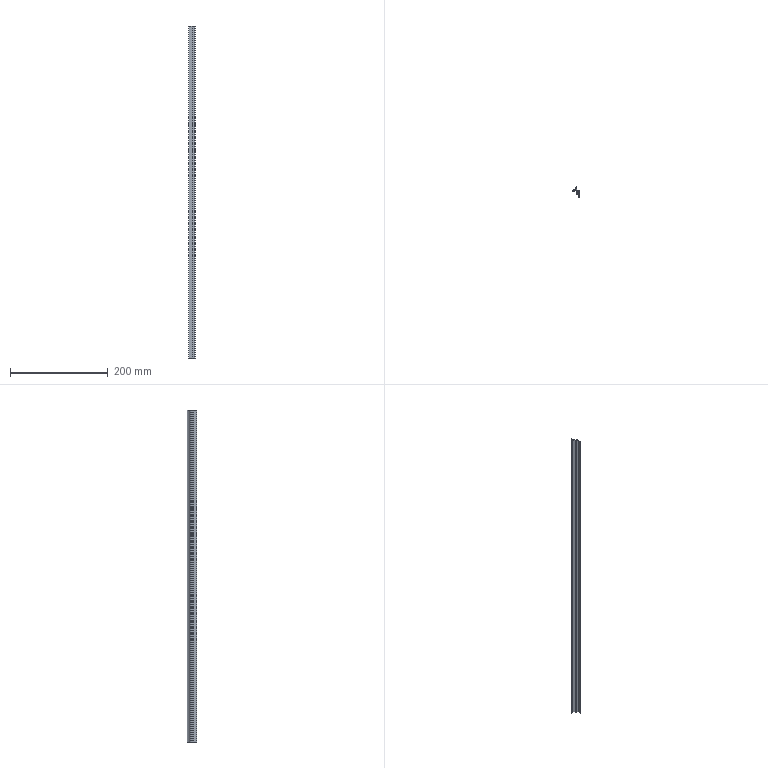Part | SolidWorks | features BaseBody 1, ICE 1, MoveFace 1 | 1 solid | 27 faces | box 14 x 20.3 x 680 mm | volume 34623 mm3 | plane 20 | cylinder 7 | commonest cylinder face diameters 0.387 x2 0.8 x2 0.4 x1 20 x1 22 x1
STEP:
#1=CARTESIAN_POINT('',(-5.304,-0.625,200.));
#2=VERTEX_POINT('',#1);
#3=CARTESIAN_POINT('',(-5.449,-0.8125,200.));
#4=VERTEX_POINT('',#3);
#5=CARTESIAN_POINT('',(-5.255,-0.8125,200.));
#6=DIRECTION('',(0.,0.,1.));
#7=DIRECTION('',(-1.,0.,0.));
#8=AXIS2_PLACEMENT_3D('',#5,#6,#7);
#9=CIRCLE('',#8,0.1937);
#10=EDGE_CURVE('',#2,#4,#9,.T.);
#11=ORIENTED_EDGE('',*,*,#10,.T.);
#12=CARTESIAN_POINT('',(-5.449,-0.8125,-480.));
#13=VERTEX_POINT('',#12);
#14=CARTESIAN_POINT('',(-5.449,-0.8125,230.));
#15=DIRECTION('',(0.,0.,-1.));
#16=VECTOR('',#15,1000.);
#17=LINE('',#14,#16);
#18=EDGE_CURVE('',#4,#13,#17,.T.);
#19=ORIENTED_EDGE('',*,*,#18,.T.);
#20=CARTESIAN_POINT('',(-5.304,-0.625,-480.));
#21=VERTEX_POINT('',#20);
#22=CARTESIAN_POINT('',(-5.255,-0.8125,-480.));
#23=DIRECTION('',(0.,0.,-1.));
#24=DIRECTION('',(1.,0.,0.));
#25=AXIS2_PLACEMENT_3D('',#22,#23,#24);
#26=CIRCLE('',#25,0.1937);
#27=EDGE_CURVE('',#13,#21,#26,.T.);
#28=ORIENTED_EDGE('',*,*,#27,.T.);
#29=CARTESIAN_POINT('',(-5.304,-0.625,230.));
#30=DIRECTION('',(0.,0.,-1.));
#31=VECTOR('',#30,1000.);
#32=LINE('',#29,#31);
#33=EDGE_CURVE('',#2,#21,#32,.T.);
#34=ORIENTED_EDGE('',*,*,#33,.F.);
#35=EDGE_LOOP('',(#11,#19,#28,#34));
#36=FACE_OUTER_BOUND('',#35,.T.);
#37=CARTESIAN_POINT('',(-5.255,-0.8125,230.));
#38=DIRECTION('',(0.,0.,-1.));
#39=DIRECTION('',(-1.,0.,0.));
#40=AXIS2_PLACEMENT_3D('',#37,#38,#39);
#41=CYLINDRICAL_SURFACE('',#40,0.1937);
#42=ADVANCED_FACE('',(#36),#41,.F.);
#43=CARTESIAN_POINT('',(5.,-1.,-480.));
#44=VERTEX_POINT('',#43);
#45=CARTESIAN_POINT('',(5.,-14.3,-480.));
#46=VERTEX_POINT('',#45);
#47=CARTESIAN_POINT('',(5.,29.623,-480.));
#48=DIRECTION('',(0.,-1.,0.));
#49=VECTOR('',#48,1000.);
#50=LINE('',#47,#49);
#51=EDGE_CURVE('',#44,#46,#50,.T.);
#52=ORIENTED_EDGE('',*,*,#51,.F.);
#53=CARTESIAN_POINT('',(5.,-1.,200.));
#54=VERTEX_POINT('',#53);
#55=CARTESIAN_POINT('',(5.,-1.,230.));
#56=DIRECTION('',(0.,0.,-1.));
#57=VECTOR('',#56,1000.);
#58=LINE('',#55,#57);
#59=EDGE_CURVE('',#54,#44,#58,.T.);
#60=ORIENTED_EDGE('',*,*,#59,.F.);
#61=CARTESIAN_POINT('',(5.,-14.3,200.));
#62=VERTEX_POINT('',#61);
#63=CARTESIAN_POINT('',(5.,-14.3,200.));
#64=DIRECTION('',(0.,1.,0.));
#65=VECTOR('',#64,1000.);
#66=LINE('',#63,#65);
#67=EDGE_CURVE('',#62,#54,#66,.T.);
#68=ORIENTED_EDGE('',*,*,#67,.F.);
#69=CARTESIAN_POINT('',(5.,-14.3,230.));
#70=DIRECTION('',(0.,0.,1.));
#71=VECTOR('',#70,1000.);
#72=LINE('',#69,#71);
#73=EDGE_CURVE('',#46,#62,#72,.T.);
#74=ORIENTED_EDGE('',*,*,#73,.F.);
#75=EDGE_LOOP('',(#52,#60,#68,#74));
#76=FACE_OUTER_BOUND('',#75,.T.);
#77=CARTESIAN_POINT('',(5.,-14.3,230.));
#78=DIRECTION('',(-1.,0.,0.));
#79=DIRECTION('',(0.,0.,1.));
#80=AXIS2_PLACEMENT_3D('',#77,#78,#79);
#81=PLANE('',#80);
#82=ADVANCED_FACE('',(#76),#81,.F.);
#83=CARTESIAN_POINT('',(-9.,-2.,-480.));
#84=VERTEX_POINT('',#83);
#85=CARTESIAN_POINT('',(-9.,-2.,200.));
#86=VERTEX_POINT('',#85);
#87=CARTESIAN_POINT('',(-9.,-2.,230.));
#88=DIRECTION('',(0.,0.,1.));
#89=VECTOR('',#88,1000.);
#90=LINE('',#87,#89);
#91=EDGE_CURVE('',#84,#86,#90,.T.);
#92=ORIENTED_EDGE('',*,*,#91,.F.);
#93=CARTESIAN_POINT('',(0.9,-2.,-480.));
#94=VERTEX_POINT('',#93);
#95=CARTESIAN_POINT('',(5.,-2.,-480.));
#96=DIRECTION('',(-1.,0.,0.));
#97=VECTOR('',#96,1000.);
#98=LINE('',#95,#97);
#99=EDGE_CURVE('',#94,#84,#98,.T.);
#100=ORIENTED_EDGE('',*,*,#99,.F.);
#101=CARTESIAN_POINT('',(0.9,-2.,200.));
#102=VERTEX_POINT('',#101);
#103=CARTESIAN_POINT('',(0.9,-2.,230.));
#104=DIRECTION('',(0.,0.,-1.));
#105=VECTOR('',#104,1000.);
#106=LINE('',#103,#105);
#107=EDGE_CURVE('',#102,#94,#106,.T.);
#108=ORIENTED_EDGE('',*,*,#107,.F.);
#109=CARTESIAN_POINT('',(5.,-2.,200.));
#110=DIRECTION('',(1.,0.,0.));
#111=VECTOR('',#110,1000.);
#112=LINE('',#109,#111);
#113=EDGE_CURVE('',#86,#102,#112,.T.);
#114=ORIENTED_EDGE('',*,*,#113,.F.);
#115=EDGE_LOOP('',(#92,#100,#108,#114));
#116=FACE_OUTER_BOUND('',#115,.T.);
#117=CARTESIAN_POINT('',(-9.,-2.,230.));
#118=DIRECTION('',(0.,1.,0.));
#119=DIRECTION('',(0.,0.,1.));
#120=AXIS2_PLACEMENT_3D('',#117,#118,#119);
#121=PLANE('',#120);
#122=ADVANCED_FACE('',(#116),#121,.F.);
#123=CARTESIAN_POINT('',(4.,-6.,200.));
#124=VERTEX_POINT('',#123);
#125=CARTESIAN_POINT('',(4.,-3.,200.));
#126=VERTEX_POINT('',#125);
#127=CARTESIAN_POINT('',(4.,29.623,200.));
#128=DIRECTION('',(0.,1.,0.));
#129=VECTOR('',#128,1000.);
#130=LINE('',#127,#129);
#131=EDGE_CURVE('',#124,#126,#130,.T.);
#132=ORIENTED_EDGE('',*,*,#131,.F.);
#133=CARTESIAN_POINT('',(1.,-6.,200.));
#134=VERTEX_POINT('',#133);
#135=CARTESIAN_POINT('',(5.,-6.,200.));
#136=DIRECTION('',(1.,0.,0.));
#137=VECTOR('',#136,1000.);
#138=LINE('',#135,#137);
#139=EDGE_CURVE('',#134,#124,#138,.T.);
#140=ORIENTED_EDGE('',*,*,#139,.F.);
#141=CARTESIAN_POINT('',(1.,-6.7,200.));
#142=VERTEX_POINT('',#141);
#143=CARTESIAN_POINT('',(1.,-6.,200.));
#144=DIRECTION('',(0.,-1.,0.));
#145=VECTOR('',#144,1000.);
#146=LINE('',#143,#145);
#147=EDGE_CURVE('',#134,#142,#146,.T.);
#148=ORIENTED_EDGE('',*,*,#147,.T.);
#149=CARTESIAN_POINT('',(-1.7,-6.7,200.));
#150=VERTEX_POINT('',#149);
#151=CARTESIAN_POINT('',(5.,-6.7,200.));
#152=DIRECTION('',(1.,0.,0.));
#153=VECTOR('',#152,1000.);
#154=LINE('',#151,#153);
#155=EDGE_CURVE('',#150,#142,#154,.T.);
#156=ORIENTED_EDGE('',*,*,#155,.F.);
#157=CARTESIAN_POINT('',(-1.7,-7.7,200.));
#158=VERTEX_POINT('',#157);
#159=CARTESIAN_POINT('',(-1.7,-6.7,200.));
#160=DIRECTION('',(0.,-1.,0.));
#161=VECTOR('',#160,1000.);
#162=LINE('',#159,#161);
#163=EDGE_CURVE('',#150,#158,#162,.T.);
#164=ORIENTED_EDGE('',*,*,#163,.T.);
#165=CARTESIAN_POINT('',(4.,-7.7,200.));
#166=VERTEX_POINT('',#165);
#167=CARTESIAN_POINT('',(5.,-7.7,200.));
#168=DIRECTION('',(-1.,0.,0.));
#169=VECTOR('',#168,1000.);
#170=LINE('',#167,#169);
#171=EDGE_CURVE('',#166,#158,#170,.T.);
#172=ORIENTED_EDGE('',*,*,#171,.F.);
#173=CARTESIAN_POINT('',(4.,-14.3,200.));
#174=VERTEX_POINT('',#173);
#175=CARTESIAN_POINT('',(4.,29.623,200.));
#176=DIRECTION('',(0.,1.,0.));
#177=VECTOR('',#176,1000.);
#178=LINE('',#175,#177);
#179=EDGE_CURVE('',#174,#166,#178,.T.);
#180=ORIENTED_EDGE('',*,*,#179,.F.);
#181=CARTESIAN_POINT('',(5.,-14.3,200.));
#182=DIRECTION('',(-1.,0.,0.));
#183=VECTOR('',#182,1000.);
#184=LINE('',#181,#183);
#185=EDGE_CURVE('',#62,#174,#184,.T.);
#186=ORIENTED_EDGE('',*,*,#185,.F.);
#187=ORIENTED_EDGE('',*,*,#67,.T.);
#188=CARTESIAN_POINT('',(-5.207,-1.,200.));
#189=VERTEX_POINT('',#188);
#190=CARTESIAN_POINT('',(5.,-1.,200.));
#191=DIRECTION('',(1.,0.,0.));
#192=VECTOR('',#191,1000.);
#193=LINE('',#190,#192);
#194=EDGE_CURVE('',#189,#54,#193,.T.);
#195=ORIENTED_EDGE('',*,*,#194,.F.);
#196=CARTESIAN_POINT('',(-5.255,-0.8125,200.));
#197=DIRECTION('',(0.,0.,1.));
#198=DIRECTION('',(-1.,0.,0.));
#199=AXIS2_PLACEMENT_3D('',#196,#197,#198);
#200=CIRCLE('',#199,0.1937);
#201=EDGE_CURVE('',#4,#189,#200,.T.);
#202=ORIENTED_EDGE('',*,*,#201,.F.);
#203=ORIENTED_EDGE('',*,*,#10,.F.);
#204=CARTESIAN_POINT('',(-1.368,3.063,200.));
#205=VERTEX_POINT('',#204);
#206=CARTESIAN_POINT('',(-10.628,9.,200.));
#207=DIRECTION('',(0.,0.,1.));
#208=DIRECTION('',(-1.,0.,0.));
#209=AXIS2_PLACEMENT_3D('',#206,#207,#208);
#210=CIRCLE('',#209,11.);
#211=EDGE_CURVE('',#2,#205,#210,.T.);
#212=ORIENTED_EDGE('',*,*,#211,.T.);
#213=CARTESIAN_POINT('',(-1.,2.955,200.));
#214=VERTEX_POINT('',#213);
#215=CARTESIAN_POINT('',(-1.2,2.955,200.));
#216=DIRECTION('',(0.,0.,1.));
#217=DIRECTION('',(-1.,0.,0.));
#218=AXIS2_PLACEMENT_3D('',#215,#216,#217);
#219=CIRCLE('',#218,0.2);
#220=EDGE_CURVE('',#214,#205,#219,.T.);
#221=ORIENTED_EDGE('',*,*,#220,.F.);
#222=CARTESIAN_POINT('',(-1.,1.5,200.));
#223=VERTEX_POINT('',#222);
#224=CARTESIAN_POINT('',(-1.,2.955,200.));
#225=DIRECTION('',(0.,1.,0.));
#226=VECTOR('',#225,1000.);
#227=LINE('',#224,#226);
#228=EDGE_CURVE('',#223,#214,#227,.T.);
#229=ORIENTED_EDGE('',*,*,#228,.F.);
#230=CARTESIAN_POINT('',(0.,1.5,200.));
#231=VERTEX_POINT('',#230);
#232=CARTESIAN_POINT('',(-1.,1.5,200.));
#233=DIRECTION('',(-1.,0.,0.));
#234=VECTOR('',#233,1000.);
#235=LINE('',#232,#234);
#236=EDGE_CURVE('',#231,#223,#235,.T.);
#237=ORIENTED_EDGE('',*,*,#236,.F.);
#238=CARTESIAN_POINT('',(0.,6.,200.));
#239=VERTEX_POINT('',#238);
#240=CARTESIAN_POINT('',(0.,1.5,200.));
#241=DIRECTION('',(0.,-1.,0.));
#242=VECTOR('',#241,1000.);
#243=LINE('',#240,#242);
#244=EDGE_CURVE('',#239,#231,#243,.T.);
#245=ORIENTED_EDGE('',*,*,#244,.F.);
#246=CARTESIAN_POINT('',(-0.8,6.,200.));
#247=VERTEX_POINT('',#246);
#248=CARTESIAN_POINT('',(0.,6.,200.));
#249=DIRECTION('',(1.,0.,0.));
#250=VECTOR('',#249,1000.);
#251=LINE('',#248,#250);
#252=EDGE_CURVE('',#247,#239,#251,.T.);
#253=ORIENTED_EDGE('',*,*,#252,.F.);
#254=CARTESIAN_POINT('',(-1.178,5.731,200.));
#255=VERTEX_POINT('',#254);
#256=CARTESIAN_POINT('',(-0.8,5.6,200.));
#257=DIRECTION('',(0.,0.,1.));
#258=DIRECTION('',(-1.,0.,0.));
#259=AXIS2_PLACEMENT_3D('',#256,#257,#258);
#260=CIRCLE('',#259,0.4);
#261=EDGE_CURVE('',#247,#255,#260,.T.);
#262=ORIENTED_EDGE('',*,*,#261,.T.);
#263=CARTESIAN_POINT('',(-8.678,-0.8077,200.));
#264=VERTEX_POINT('',#263);
#265=CARTESIAN_POINT('',(-10.628,9.,200.));
#266=DIRECTION('',(0.,0.,1.));
#267=DIRECTION('',(-1.,0.,0.));
#268=AXIS2_PLACEMENT_3D('',#265,#266,#267);
#269=CIRCLE('',#268,10.);
#270=EDGE_CURVE('',#264,#255,#269,.T.);
#271=ORIENTED_EDGE('',*,*,#270,.F.);
#272=CARTESIAN_POINT('',(-9.,-1.2,200.));
#273=VERTEX_POINT('',#272);
#274=CARTESIAN_POINT('',(-8.6,-1.2,200.));
#275=DIRECTION('',(0.,0.,1.));
#276=DIRECTION('',(-1.,0.,0.));
#277=AXIS2_PLACEMENT_3D('',#274,#275,#276);
#278=CIRCLE('',#277,0.4);
#279=EDGE_CURVE('',#264,#273,#278,.T.);
#280=ORIENTED_EDGE('',*,*,#279,.T.);
#281=CARTESIAN_POINT('',(-9.,8.,200.));
#282=DIRECTION('',(0.,-1.,0.));
#283=VECTOR('',#282,1000.);
#284=LINE('',#281,#283);
#285=EDGE_CURVE('',#273,#86,#284,.T.);
#286=ORIENTED_EDGE('',*,*,#285,.T.);
#287=ORIENTED_EDGE('',*,*,#113,.T.);
#288=CARTESIAN_POINT('',(0.9,-3.,200.));
#289=VERTEX_POINT('',#288);
#290=CARTESIAN_POINT('',(0.9,29.623,200.));
#291=DIRECTION('',(0.,1.,0.));
#292=VECTOR('',#291,1000.);
#293=LINE('',#290,#292);
#294=EDGE_CURVE('',#289,#102,#293,.T.);
#295=ORIENTED_EDGE('',*,*,#294,.F.);
#296=CARTESIAN_POINT('',(5.,-3.,200.));
#297=DIRECTION('',(-1.,0.,0.));
#298=VECTOR('',#297,1000.);
#299=LINE('',#296,#298);
#300=EDGE_CURVE('',#126,#289,#299,.T.);
#301=ORIENTED_EDGE('',*,*,#300,.F.);
#302=EDGE_LOOP('',(#132,#140,#148,#156,#164,#172,#180,#186,#187,#195,#202,#203,#212,#221,#229,#237,#245,#253,#262,#271,#280,#286,#287,#295,#301));
#303=FACE_OUTER_BOUND('',#302,.T.);
#304=CARTESIAN_POINT('',(5.,29.623,200.));
#305=DIRECTION('',(0.,0.,-1.));
#306=DIRECTION('',(-1.,0.,0.));
#307=AXIS2_PLACEMENT_3D('',#304,#305,#306);
#308=PLANE('',#307);
#309=ADVANCED_FACE('',(#303),#308,.F.);
#310=ORIENTED_EDGE('',*,*,#185,.T.);
#311=CARTESIAN_POINT('',(4.,-14.3,-480.));
#312=VERTEX_POINT('',#311);
#313=CARTESIAN_POINT('',(4.,-14.3,230.));
#314=DIRECTION('',(0.,0.,1.));
#315=VECTOR('',#314,1000.);
#316=LINE('',#313,#315);
#317=EDGE_CURVE('',#312,#174,#316,.T.);
#318=ORIENTED_EDGE('',*,*,#317,.F.);
#319=CARTESIAN_POINT('',(5.,-14.3,-480.));
#320=DIRECTION('',(-1.,0.,0.));
#321=VECTOR('',#320,1000.);
#322=LINE('',#319,#321);
#323=EDGE_CURVE('',#46,#312,#322,.T.);
#324=ORIENTED_EDGE('',*,*,#323,.F.);
#325=ORIENTED_EDGE('',*,*,#73,.T.);
#326=EDGE_LOOP('',(#310,#318,#324,#325));
#327=FACE_OUTER_BOUND('',#326,.T.);
#328=CARTESIAN_POINT('',(4.,-14.3,230.));
#329=DIRECTION('',(0.,1.,0.));
#330=DIRECTION('',(0.,0.,1.));
#331=AXIS2_PLACEMENT_3D('',#328,#329,#330);
#332=PLANE('',#331);
#333=ADVANCED_FACE('',(#327),#332,.F.);
#334=ORIENTED_EDGE('',*,*,#51,.T.);
#335=ORIENTED_EDGE('',*,*,#323,.T.);
#336=CARTESIAN_POINT('',(4.,-7.7,-480.));
#337=VERTEX_POINT('',#336);
#338=CARTESIAN_POINT('',(4.,-7.7,-480.));
#339=DIRECTION('',(0.,-1.,0.));
#340=VECTOR('',#339,1000.);
#341=LINE('',#338,#340);
#342=EDGE_CURVE('',#337,#312,#341,.T.);
#343=ORIENTED_EDGE('',*,*,#342,.F.);
#344=CARTESIAN_POINT('',(-1.7,-7.7,-480.));
#345=VERTEX_POINT('',#344);
#346=CARTESIAN_POINT('',(-1.7,-7.7,-480.));
#347=DIRECTION('',(1.,0.,0.));
#348=VECTOR('',#347,1000.);
#349=LINE('',#346,#348);
#350=EDGE_CURVE('',#345,#337,#349,.T.);
#351=ORIENTED_EDGE('',*,*,#350,.F.);
#352=CARTESIAN_POINT('',(-1.7,-6.7,-480.));
#353=VERTEX_POINT('',#352);
#354=CARTESIAN_POINT('',(-1.7,29.623,-480.));
#355=DIRECTION('',(0.,1.,0.));
#356=VECTOR('',#355,1000.);
#357=LINE('',#354,#356);
#358=EDGE_CURVE('',#345,#353,#357,.T.);
#359=ORIENTED_EDGE('',*,*,#358,.T.);
#360=CARTESIAN_POINT('',(1.,-6.7,-480.));
#361=VERTEX_POINT('',#360);
#362=CARTESIAN_POINT('',(1.,-6.7,-480.));
#363=DIRECTION('',(-1.,0.,0.));
#364=VECTOR('',#363,1000.);
#365=LINE('',#362,#364);
#366=EDGE_CURVE('',#361,#353,#365,.T.);
#367=ORIENTED_EDGE('',*,*,#366,.F.);
#368=CARTESIAN_POINT('',(1.,-6.,-480.));
#369=VERTEX_POINT('',#368);
#370=CARTESIAN_POINT('',(1.,29.623,-480.));
#371=DIRECTION('',(0.,1.,0.));
#372=VECTOR('',#371,1000.);
#373=LINE('',#370,#372);
#374=EDGE_CURVE('',#361,#369,#373,.T.);
#375=ORIENTED_EDGE('',*,*,#374,.T.);
#376=CARTESIAN_POINT('',(4.,-6.,-480.));
#377=VERTEX_POINT('',#376);
#378=CARTESIAN_POINT('',(4.,-6.,-480.));
#379=DIRECTION('',(-1.,0.,0.));
#380=VECTOR('',#379,1000.);
#381=LINE('',#378,#380);
#382=EDGE_CURVE('',#377,#369,#381,.T.);
#383=ORIENTED_EDGE('',*,*,#382,.F.);
#384=CARTESIAN_POINT('',(4.,-3.,-480.));
#385=VERTEX_POINT('',#384);
#386=CARTESIAN_POINT('',(4.,-3.,-480.));
#387=DIRECTION('',(0.,-1.,0.));
#388=VECTOR('',#387,1000.);
#389=LINE('',#386,#388);
#390=EDGE_CURVE('',#385,#377,#389,.T.);
#391=ORIENTED_EDGE('',*,*,#390,.F.);
#392=CARTESIAN_POINT('',(0.9,-3.,-480.));
#393=VERTEX_POINT('',#392);
#394=CARTESIAN_POINT('',(0.9,-3.,-480.));
#395=DIRECTION('',(1.,0.,0.));
#396=VECTOR('',#395,1000.);
#397=LINE('',#394,#396);
#398=EDGE_CURVE('',#393,#385,#397,.T.);
#399=ORIENTED_EDGE('',*,*,#398,.F.);
#400=CARTESIAN_POINT('',(0.9,-2.,-480.));
#401=DIRECTION('',(0.,-1.,0.));
#402=VECTOR('',#401,1000.);
#403=LINE('',#400,#402);
#404=EDGE_CURVE('',#94,#393,#403,.T.);
#405=ORIENTED_EDGE('',*,*,#404,.F.);
#406=ORIENTED_EDGE('',*,*,#99,.T.);
#407=CARTESIAN_POINT('',(-9.,-1.2,-480.));
#408=VERTEX_POINT('',#407);
#409=CARTESIAN_POINT('',(-9.,-1.2,-480.));
#410=DIRECTION('',(0.,-1.,0.));
#411=VECTOR('',#410,1000.);
#412=LINE('',#409,#411);
#413=EDGE_CURVE('',#408,#84,#412,.T.);
#414=ORIENTED_EDGE('',*,*,#413,.F.);
#415=CARTESIAN_POINT('',(-8.678,-0.8077,-480.));
#416=VERTEX_POINT('',#415);
#417=CARTESIAN_POINT('',(-8.6,-1.2,-480.));
#418=DIRECTION('',(0.,0.,-1.));
#419=DIRECTION('',(1.,0.,0.));
#420=AXIS2_PLACEMENT_3D('',#417,#418,#419);
#421=CIRCLE('',#420,0.4);
#422=EDGE_CURVE('',#408,#416,#421,.T.);
#423=ORIENTED_EDGE('',*,*,#422,.T.);
#424=CARTESIAN_POINT('',(-1.178,5.731,-480.));
#425=VERTEX_POINT('',#424);
#426=CARTESIAN_POINT('',(-10.628,9.,-480.));
#427=DIRECTION('',(0.,0.,-1.));
#428=DIRECTION('',(1.,0.,0.));
#429=AXIS2_PLACEMENT_3D('',#426,#427,#428);
#430=CIRCLE('',#429,10.);
#431=EDGE_CURVE('',#425,#416,#430,.T.);
#432=ORIENTED_EDGE('',*,*,#431,.F.);
#433=CARTESIAN_POINT('',(-0.8,6.,-480.));
#434=VERTEX_POINT('',#433);
#435=CARTESIAN_POINT('',(-0.8,5.6,-480.));
#436=DIRECTION('',(0.,0.,-1.));
#437=DIRECTION('',(1.,0.,0.));
#438=AXIS2_PLACEMENT_3D('',#435,#436,#437);
#439=CIRCLE('',#438,0.4);
#440=EDGE_CURVE('',#425,#434,#439,.T.);
#441=ORIENTED_EDGE('',*,*,#440,.T.);
#442=CARTESIAN_POINT('',(0.,6.,-480.));
#443=VERTEX_POINT('',#442);
#444=CARTESIAN_POINT('',(0.,6.,-480.));
#445=DIRECTION('',(-1.,0.,0.));
#446=VECTOR('',#445,1000.);
#447=LINE('',#444,#446);
#448=EDGE_CURVE('',#443,#434,#447,.T.);
#449=ORIENTED_EDGE('',*,*,#448,.F.);
#450=CARTESIAN_POINT('',(0.,1.5,-480.));
#451=VERTEX_POINT('',#450);
#452=CARTESIAN_POINT('',(0.,1.5,-480.));
#453=DIRECTION('',(0.,1.,0.));
#454=VECTOR('',#453,1000.);
#455=LINE('',#452,#454);
#456=EDGE_CURVE('',#451,#443,#455,.T.);
#457=ORIENTED_EDGE('',*,*,#456,.F.);
#458=CARTESIAN_POINT('',(-1.,1.5,-480.));
#459=VERTEX_POINT('',#458);
#460=CARTESIAN_POINT('',(-1.,1.5,-480.));
#461=DIRECTION('',(1.,0.,0.));
#462=VECTOR('',#461,1000.);
#463=LINE('',#460,#462);
#464=EDGE_CURVE('',#459,#451,#463,.T.);
#465=ORIENTED_EDGE('',*,*,#464,.F.);
#466=CARTESIAN_POINT('',(-1.,2.955,-480.));
#467=VERTEX_POINT('',#466);
#468=CARTESIAN_POINT('',(-1.,2.955,-480.));
#469=DIRECTION('',(0.,-1.,0.));
#470=VECTOR('',#469,1000.);
#471=LINE('',#468,#470);
#472=EDGE_CURVE('',#467,#459,#471,.T.);
#473=ORIENTED_EDGE('',*,*,#472,.F.);
#474=CARTESIAN_POINT('',(-1.368,3.063,-480.));
#475=VERTEX_POINT('',#474);
#476=CARTESIAN_POINT('',(-1.2,2.955,-480.));
#477=DIRECTION('',(0.,0.,-1.));
#478=DIRECTION('',(1.,0.,0.));
#479=AXIS2_PLACEMENT_3D('',#476,#477,#478);
#480=CIRCLE('',#479,0.2);
#481=EDGE_CURVE('',#475,#467,#480,.T.);
#482=ORIENTED_EDGE('',*,*,#481,.F.);
#483=CARTESIAN_POINT('',(-10.628,9.,-480.));
#484=DIRECTION('',(0.,0.,-1.));
#485=DIRECTION('',(1.,0.,0.));
#486=AXIS2_PLACEMENT_3D('',#483,#484,#485);
#487=CIRCLE('',#486,11.);
#488=EDGE_CURVE('',#475,#21,#487,.T.);
#489=ORIENTED_EDGE('',*,*,#488,.T.);
#490=ORIENTED_EDGE('',*,*,#27,.F.);
#491=CARTESIAN_POINT('',(-5.207,-1.,-480.));
#492=VERTEX_POINT('',#491);
#493=CARTESIAN_POINT('',(-5.255,-0.8125,-480.));
#494=DIRECTION('',(0.,0.,-1.));
#495=DIRECTION('',(1.,0.,0.));
#496=AXIS2_PLACEMENT_3D('',#493,#494,#495);
#497=CIRCLE('',#496,0.1937);
#498=EDGE_CURVE('',#492,#13,#497,.T.);
#499=ORIENTED_EDGE('',*,*,#498,.F.);
#500=CARTESIAN_POINT('',(5.,-1.,-480.));
#501=DIRECTION('',(-1.,0.,0.));
#502=VECTOR('',#501,1000.);
#503=LINE('',#500,#502);
#504=EDGE_CURVE('',#44,#492,#503,.T.);
#505=ORIENTED_EDGE('',*,*,#504,.F.);
#506=EDGE_LOOP('',(#334,#335,#343,#351,#359,#367,#375,#383,#391,#399,#405,#406,#414,#423,#432,#441,#449,#457,#465,#473,#482,#489,#490,#499,#505));
#507=FACE_OUTER_BOUND('',#506,.T.);
#508=CARTESIAN_POINT('',(5.,29.623,-480.));
#509=DIRECTION('',(0.,0.,1.));
#510=DIRECTION('',(1.,0.,0.));
#511=AXIS2_PLACEMENT_3D('',#508,#509,#510);
#512=PLANE('',#511);
#513=ADVANCED_FACE('',(#507),#512,.F.);
#514=ORIENTED_EDGE('',*,*,#59,.T.);
#515=ORIENTED_EDGE('',*,*,#504,.T.);
#516=CARTESIAN_POINT('',(-5.207,-1.,230.));
#517=DIRECTION('',(0.,0.,-1.));
#518=VECTOR('',#517,1000.);
#519=LINE('',#516,#518);
#520=EDGE_CURVE('',#189,#492,#519,.T.);
#521=ORIENTED_EDGE('',*,*,#520,.F.);
#522=ORIENTED_EDGE('',*,*,#194,.T.);
#523=EDGE_LOOP('',(#514,#515,#521,#522));
#524=FACE_OUTER_BOUND('',#523,.T.);
#525=CARTESIAN_POINT('',(5.,-1.,230.));
#526=DIRECTION('',(0.,-1.,0.));
#527=DIRECTION('',(0.,0.,-1.));
#528=AXIS2_PLACEMENT_3D('',#525,#526,#527);
#529=PLANE('',#528);
#530=ADVANCED_FACE('',(#524),#529,.F.);
#531=CARTESIAN_POINT('',(-9.,-1.2,230.));
#532=DIRECTION('',(0.,0.,1.));
#533=VECTOR('',#532,1000.);
#534=LINE('',#531,#533);
#535=EDGE_CURVE('',#408,#273,#534,.T.);
#536=ORIENTED_EDGE('',*,*,#535,.F.);
#537=ORIENTED_EDGE('',*,*,#413,.T.);
#538=ORIENTED_EDGE('',*,*,#91,.T.);
#539=ORIENTED_EDGE('',*,*,#285,.F.);
#540=EDGE_LOOP('',(#536,#537,#538,#539));
#541=FACE_OUTER_BOUND('',#540,.T.);
#542=CARTESIAN_POINT('',(-9.,-1.2,230.));
#543=DIRECTION('',(1.,0.,0.));
#544=DIRECTION('',(0.,0.,-1.));
#545=AXIS2_PLACEMENT_3D('',#542,#543,#544);
#546=PLANE('',#545);
#547=ADVANCED_FACE('',(#541),#546,.F.);
#548=ORIENTED_EDGE('',*,*,#294,.T.);
#549=ORIENTED_EDGE('',*,*,#107,.T.);
#550=ORIENTED_EDGE('',*,*,#404,.T.);
#551=CARTESIAN_POINT('',(0.9,-3.,230.));
#552=DIRECTION('',(0.,0.,-1.));
#553=VECTOR('',#552,1000.);
#554=LINE('',#551,#553);
#555=EDGE_CURVE('',#289,#393,#554,.T.);
#556=ORIENTED_EDGE('',*,*,#555,.F.);
#557=EDGE_LOOP('',(#548,#549,#550,#556));
#558=FACE_OUTER_BOUND('',#557,.T.);
#559=CARTESIAN_POINT('',(0.9,-2.,230.));
#560=DIRECTION('',(1.,0.,0.));
#561=DIRECTION('',(0.,0.,-1.));
#562=AXIS2_PLACEMENT_3D('',#559,#560,#561);
#563=PLANE('',#562);
#564=ADVANCED_FACE('',(#558),#563,.F.);
#565=ORIENTED_EDGE('',*,*,#300,.T.);
#566=ORIENTED_EDGE('',*,*,#555,.T.);
#567=ORIENTED_EDGE('',*,*,#398,.T.);
#568=CARTESIAN_POINT('',(4.,-3.,230.));
#569=DIRECTION('',(0.,0.,-1.));
#570=VECTOR('',#569,1000.);
#571=LINE('',#568,#570);
#572=EDGE_CURVE('',#126,#385,#571,.T.);
#573=ORIENTED_EDGE('',*,*,#572,.F.);
#574=EDGE_LOOP('',(#565,#566,#567,#573));
#575=FACE_OUTER_BOUND('',#574,.T.);
#576=CARTESIAN_POINT('',(0.9,-3.,230.));
#577=DIRECTION('',(0.,1.,0.));
#578=DIRECTION('',(0.,0.,1.));
#579=AXIS2_PLACEMENT_3D('',#576,#577,#578);
#580=PLANE('',#579);
#581=ADVANCED_FACE('',(#575),#580,.F.);
#582=ORIENTED_EDGE('',*,*,#131,.T.);
#583=ORIENTED_EDGE('',*,*,#572,.T.);
#584=ORIENTED_EDGE('',*,*,#390,.T.);
#585=CARTESIAN_POINT('',(4.,-6.,230.));
#586=DIRECTION('',(0.,0.,-1.));
#587=VECTOR('',#586,1000.);
#588=LINE('',#585,#587);
#589=EDGE_CURVE('',#124,#377,#588,.T.);
#590=ORIENTED_EDGE('',*,*,#589,.F.);
#591=EDGE_LOOP('',(#582,#583,#584,#590));
#592=FACE_OUTER_BOUND('',#591,.T.);
#593=CARTESIAN_POINT('',(4.,-3.,230.));
#594=DIRECTION('',(1.,0.,0.));
#595=DIRECTION('',(0.,0.,-1.));
#596=AXIS2_PLACEMENT_3D('',#593,#594,#595);
#597=PLANE('',#596);
#598=ADVANCED_FACE('',(#592),#597,.F.);
#599=ORIENTED_EDGE('',*,*,#139,.T.);
#600=ORIENTED_EDGE('',*,*,#589,.T.);
#601=ORIENTED_EDGE('',*,*,#382,.T.);
#602=CARTESIAN_POINT('',(1.,-6.,230.));
#603=DIRECTION('',(0.,0.,-1.));
#604=VECTOR('',#603,1000.);
#605=LINE('',#602,#604);
#606=EDGE_CURVE('',#134,#369,#605,.T.);
#607=ORIENTED_EDGE('',*,*,#606,.F.);
#608=EDGE_LOOP('',(#599,#600,#601,#607));
#609=FACE_OUTER_BOUND('',#608,.T.);
#610=CARTESIAN_POINT('',(4.,-6.,230.));
#611=DIRECTION('',(0.,-1.,0.));
#612=DIRECTION('',(0.,0.,-1.));
#613=AXIS2_PLACEMENT_3D('',#610,#611,#612);
#614=PLANE('',#613);
#615=ADVANCED_FACE('',(#609),#614,.F.);
#616=ORIENTED_EDGE('',*,*,#155,.T.);
#617=CARTESIAN_POINT('',(1.,-6.7,230.));
#618=DIRECTION('',(0.,0.,1.));
#619=VECTOR('',#618,1000.);
#620=LINE('',#617,#619);
#621=EDGE_CURVE('',#361,#142,#620,.T.);
#622=ORIENTED_EDGE('',*,*,#621,.F.);
#623=ORIENTED_EDGE('',*,*,#366,.T.);
#624=CARTESIAN_POINT('',(-1.7,-6.7,230.));
#625=DIRECTION('',(0.,0.,-1.));
#626=VECTOR('',#625,1000.);
#627=LINE('',#624,#626);
#628=EDGE_CURVE('',#150,#353,#627,.T.);
#629=ORIENTED_EDGE('',*,*,#628,.F.);
#630=EDGE_LOOP('',(#616,#622,#623,#629));
#631=FACE_OUTER_BOUND('',#630,.T.);
#632=CARTESIAN_POINT('',(1.,-6.7,230.));
#633=DIRECTION('',(0.,-1.,0.));
#634=DIRECTION('',(0.,0.,-1.));
#635=AXIS2_PLACEMENT_3D('',#632,#633,#634);
#636=PLANE('',#635);
#637=ADVANCED_FACE('',(#631),#636,.F.);
#638=ORIENTED_EDGE('',*,*,#171,.T.);
#639=CARTESIAN_POINT('',(-1.7,-7.7,230.));
#640=DIRECTION('',(0.,0.,1.));
#641=VECTOR('',#640,1000.);
#642=LINE('',#639,#641);
#643=EDGE_CURVE('',#345,#158,#642,.T.);
#644=ORIENTED_EDGE('',*,*,#643,.F.);
#645=ORIENTED_EDGE('',*,*,#350,.T.);
#646=CARTESIAN_POINT('',(4.,-7.7,230.));
#647=DIRECTION('',(0.,0.,-1.));
#648=VECTOR('',#647,1000.);
#649=LINE('',#646,#648);
#650=EDGE_CURVE('',#166,#337,#649,.T.);
#651=ORIENTED_EDGE('',*,*,#650,.F.);
#652=EDGE_LOOP('',(#638,#644,#645,#651));
#653=FACE_OUTER_BOUND('',#652,.T.);
#654=CARTESIAN_POINT('',(-1.7,-7.7,230.));
#655=DIRECTION('',(0.,1.,0.));
#656=DIRECTION('',(0.,0.,1.));
#657=AXIS2_PLACEMENT_3D('',#654,#655,#656);
#658=PLANE('',#657);
#659=ADVANCED_FACE('',(#653),#658,.F.);
#660=ORIENTED_EDGE('',*,*,#179,.T.);
#661=ORIENTED_EDGE('',*,*,#650,.T.);
#662=ORIENTED_EDGE('',*,*,#342,.T.);
#663=ORIENTED_EDGE('',*,*,#317,.T.);
#664=EDGE_LOOP('',(#660,#661,#662,#663));
#665=FACE_OUTER_BOUND('',#664,.T.);
#666=CARTESIAN_POINT('',(4.,-7.7,230.));
#667=DIRECTION('',(1.,0.,0.));
#668=DIRECTION('',(0.,0.,-1.));
#669=AXIS2_PLACEMENT_3D('',#666,#667,#668);
#670=PLANE('',#669);
#671=ADVANCED_FACE('',(#665),#670,.F.);
#672=ORIENTED_EDGE('',*,*,#18,.F.);
#673=ORIENTED_EDGE('',*,*,#201,.T.);
#674=ORIENTED_EDGE('',*,*,#520,.T.);
#675=ORIENTED_EDGE('',*,*,#498,.T.);
#676=EDGE_LOOP('',(#672,#673,#674,#675));
#677=FACE_OUTER_BOUND('',#676,.T.);
#678=CARTESIAN_POINT('',(-5.255,-0.8125,230.));
#679=DIRECTION('',(0.,0.,-1.));
#680=DIRECTION('',(-1.,0.,0.));
#681=AXIS2_PLACEMENT_3D('',#678,#679,#680);
#682=CYLINDRICAL_SURFACE('',#681,0.1937);
#683=ADVANCED_FACE('',(#677),#682,.F.);
#684=CARTESIAN_POINT('',(-1.,2.955,230.));
#685=DIRECTION('',(0.,0.,1.));
#686=VECTOR('',#685,1000.);
#687=LINE('',#684,#686);
#688=EDGE_CURVE('',#467,#214,#687,.T.);
#689=ORIENTED_EDGE('',*,*,#688,.F.);
#690=ORIENTED_EDGE('',*,*,#472,.T.);
#691=CARTESIAN_POINT('',(-1.,1.5,230.));
#692=DIRECTION('',(0.,0.,-1.));
#693=VECTOR('',#692,1000.);
#694=LINE('',#691,#693);
#695=EDGE_CURVE('',#223,#459,#694,.T.);
#696=ORIENTED_EDGE('',*,*,#695,.F.);
#697=ORIENTED_EDGE('',*,*,#228,.T.);
#698=EDGE_LOOP('',(#689,#690,#696,#697));
#699=FACE_OUTER_BOUND('',#698,.T.);
#700=CARTESIAN_POINT('',(-1.,2.955,230.));
#701=DIRECTION('',(1.,0.,0.));
#702=DIRECTION('',(0.,0.,-1.));
#703=AXIS2_PLACEMENT_3D('',#700,#701,#702);
#704=PLANE('',#703);
#705=ADVANCED_FACE('',(#699),#704,.F.);
#706=ORIENTED_EDGE('',*,*,#488,.F.);
#707=CARTESIAN_POINT('',(-1.368,3.063,230.));
#708=DIRECTION('',(0.,0.,1.));
#709=VECTOR('',#708,1000.);
#710=LINE('',#707,#709);
#711=EDGE_CURVE('',#475,#205,#710,.T.);
#712=ORIENTED_EDGE('',*,*,#711,.T.);
#713=ORIENTED_EDGE('',*,*,#211,.F.);
#714=ORIENTED_EDGE('',*,*,#33,.T.);
#715=EDGE_LOOP('',(#706,#712,#713,#714));
#716=FACE_OUTER_BOUND('',#715,.T.);
#717=CARTESIAN_POINT('',(-10.628,9.,230.));
#718=DIRECTION('',(0.,0.,-1.));
#719=DIRECTION('',(-1.,0.,0.));
#720=AXIS2_PLACEMENT_3D('',#717,#718,#719);
#721=CYLINDRICAL_SURFACE('',#720,11.);
#722=ADVANCED_FACE('',(#716),#721,.T.);
#723=CARTESIAN_POINT('',(-1.178,5.731,230.));
#724=DIRECTION('',(0.,0.,1.));
#725=VECTOR('',#724,1000.);
#726=LINE('',#723,#725);
#727=EDGE_CURVE('',#425,#255,#726,.T.);
#728=ORIENTED_EDGE('',*,*,#727,.F.);
#729=ORIENTED_EDGE('',*,*,#431,.T.);
#730=CARTESIAN_POINT('',(-8.678,-0.8077,230.));
#731=DIRECTION('',(0.,0.,-1.));
#732=VECTOR('',#731,1000.);
#733=LINE('',#730,#732);
#734=EDGE_CURVE('',#264,#416,#733,.T.);
#735=ORIENTED_EDGE('',*,*,#734,.F.);
#736=ORIENTED_EDGE('',*,*,#270,.T.);
#737=EDGE_LOOP('',(#728,#729,#735,#736));
#738=FACE_OUTER_BOUND('',#737,.T.);
#739=CARTESIAN_POINT('',(-10.628,9.,230.));
#740=DIRECTION('',(0.,0.,-1.));
#741=DIRECTION('',(-1.,0.,0.));
#742=AXIS2_PLACEMENT_3D('',#739,#740,#741);
#743=CYLINDRICAL_SURFACE('',#742,10.);
#744=ADVANCED_FACE('',(#738),#743,.F.);
#745=CARTESIAN_POINT('',(0.,1.5,230.));
#746=DIRECTION('',(0.,0.,1.));
#747=VECTOR('',#746,1000.);
#748=LINE('',#745,#747);
#749=EDGE_CURVE('',#451,#231,#748,.T.);
#750=ORIENTED_EDGE('',*,*,#749,.F.);
#751=ORIENTED_EDGE('',*,*,#456,.T.);
#752=CARTESIAN_POINT('',(0.,6.,230.));
#753=DIRECTION('',(0.,0.,-1.));
#754=VECTOR('',#753,1000.);
#755=LINE('',#752,#754);
#756=EDGE_CURVE('',#239,#443,#755,.T.);
#757=ORIENTED_EDGE('',*,*,#756,.F.);
#758=ORIENTED_EDGE('',*,*,#244,.T.);
#759=EDGE_LOOP('',(#750,#751,#757,#758));
#760=FACE_OUTER_BOUND('',#759,.T.);
#761=CARTESIAN_POINT('',(0.,1.5,230.));
#762=DIRECTION('',(-1.,0.,0.));
#763=DIRECTION('',(0.,0.,1.));
#764=AXIS2_PLACEMENT_3D('',#761,#762,#763);
#765=PLANE('',#764);
#766=ADVANCED_FACE('',(#760),#765,.F.);
#767=ORIENTED_EDGE('',*,*,#422,.F.);
#768=ORIENTED_EDGE('',*,*,#535,.T.);
#769=ORIENTED_EDGE('',*,*,#279,.F.);
#770=ORIENTED_EDGE('',*,*,#734,.T.);
#771=EDGE_LOOP('',(#767,#768,#769,#770));
#772=FACE_OUTER_BOUND('',#771,.T.);
#773=CARTESIAN_POINT('',(-8.6,-1.2,230.));
#774=DIRECTION('',(0.,0.,-1.));
#775=DIRECTION('',(-1.,0.,0.));
#776=AXIS2_PLACEMENT_3D('',#773,#774,#775);
#777=CYLINDRICAL_SURFACE('',#776,0.4);
#778=ADVANCED_FACE('',(#772),#777,.T.);
#779=ORIENTED_EDGE('',*,*,#147,.F.);
#780=ORIENTED_EDGE('',*,*,#606,.T.);
#781=ORIENTED_EDGE('',*,*,#374,.F.);
#782=ORIENTED_EDGE('',*,*,#621,.T.);
#783=EDGE_LOOP('',(#779,#780,#781,#782));
#784=FACE_OUTER_BOUND('',#783,.T.);
#785=CARTESIAN_POINT('',(1.,-6.,230.));
#786=DIRECTION('',(1.,0.,0.));
#787=DIRECTION('',(0.,0.,-1.));
#788=AXIS2_PLACEMENT_3D('',#785,#786,#787);
#789=PLANE('',#788);
#790=ADVANCED_FACE('',(#784),#789,.F.);
#791=ORIENTED_EDGE('',*,*,#163,.F.);
#792=ORIENTED_EDGE('',*,*,#628,.T.);
#793=ORIENTED_EDGE('',*,*,#358,.F.);
#794=ORIENTED_EDGE('',*,*,#643,.T.);
#795=EDGE_LOOP('',(#791,#792,#793,#794));
#796=FACE_OUTER_BOUND('',#795,.T.);
#797=CARTESIAN_POINT('',(-1.7,-6.7,230.));
#798=DIRECTION('',(1.,0.,0.));
#799=DIRECTION('',(0.,0.,-1.));
#800=AXIS2_PLACEMENT_3D('',#797,#798,#799);
#801=PLANE('',#800);
#802=ADVANCED_FACE('',(#796),#801,.F.);
#803=ORIENTED_EDGE('',*,*,#711,.F.);
#804=ORIENTED_EDGE('',*,*,#481,.T.);
#805=ORIENTED_EDGE('',*,*,#688,.T.);
#806=ORIENTED_EDGE('',*,*,#220,.T.);
#807=EDGE_LOOP('',(#803,#804,#805,#806));
#808=FACE_OUTER_BOUND('',#807,.T.);
#809=CARTESIAN_POINT('',(-1.2,2.955,230.));
#810=DIRECTION('',(0.,0.,-1.));
#811=DIRECTION('',(-1.,0.,0.));
#812=AXIS2_PLACEMENT_3D('',#809,#810,#811);
#813=CYLINDRICAL_SURFACE('',#812,0.2);
#814=ADVANCED_FACE('',(#808),#813,.F.);
#815=ORIENTED_EDGE('',*,*,#695,.T.);
#816=ORIENTED_EDGE('',*,*,#464,.T.);
#817=ORIENTED_EDGE('',*,*,#749,.T.);
#818=ORIENTED_EDGE('',*,*,#236,.T.);
#819=EDGE_LOOP('',(#815,#816,#817,#818));
#820=FACE_OUTER_BOUND('',#819,.T.);
#821=CARTESIAN_POINT('',(-1.,1.5,230.));
#822=DIRECTION('',(0.,1.,0.));
#823=DIRECTION('',(0.,0.,1.));
#824=AXIS2_PLACEMENT_3D('',#821,#822,#823);
#825=PLANE('',#824);
#826=ADVANCED_FACE('',(#820),#825,.F.);
#827=ORIENTED_EDGE('',*,*,#440,.F.);
#828=ORIENTED_EDGE('',*,*,#727,.T.);
#829=ORIENTED_EDGE('',*,*,#261,.F.);
#830=CARTESIAN_POINT('',(-0.8,6.,230.));
#831=DIRECTION('',(0.,0.,-1.));
#832=VECTOR('',#831,1000.);
#833=LINE('',#830,#832);
#834=EDGE_CURVE('',#247,#434,#833,.T.);
#835=ORIENTED_EDGE('',*,*,#834,.T.);
#836=EDGE_LOOP('',(#827,#828,#829,#835));
#837=FACE_OUTER_BOUND('',#836,.T.);
#838=CARTESIAN_POINT('',(-0.8,5.6,230.));
#839=DIRECTION('',(0.,0.,-1.));
#840=DIRECTION('',(-1.,0.,0.));
#841=AXIS2_PLACEMENT_3D('',#838,#839,#840);
#842=CYLINDRICAL_SURFACE('',#841,0.4);
#843=ADVANCED_FACE('',(#837),#842,.T.);
#844=ORIENTED_EDGE('',*,*,#756,.T.);
#845=ORIENTED_EDGE('',*,*,#448,.T.);
#846=ORIENTED_EDGE('',*,*,#834,.F.);
#847=ORIENTED_EDGE('',*,*,#252,.T.);
#848=EDGE_LOOP('',(#844,#845,#846,#847));
#849=FACE_OUTER_BOUND('',#848,.T.);
#850=CARTESIAN_POINT('',(0.,6.,230.));
#851=DIRECTION('',(0.,-1.,0.));
#852=DIRECTION('',(0.,0.,-1.));
#853=AXIS2_PLACEMENT_3D('',#850,#851,#852);
#854=PLANE('',#853);
#855=ADVANCED_FACE('',(#849),#854,.F.);
#856=CLOSED_SHELL('',(#42,#82,#122,#309,#333,#513,#530,#547,#564,#581,#598,#615,#637,#659,#671,#683,#705,#722,#744,#766,#778,#790,#802,#814,#826,#843,#855));
#857=MANIFOLD_SOLID_BREP('',#856);
#858=CARTESIAN_POINT('',(0.,0.,0.));
#859=DIRECTION('',(0.,0.,1.));
#860=DIRECTION('',(1.,0.,0.));
#861=AXIS2_PLACEMENT_3D('',#858,#859,#860);
#862=(LENGTH_UNIT()NAMED_UNIT(*)SI_UNIT(.MILLI.,.METRE.));
#863=UNCERTAINTY_MEASURE_WITH_UNIT(LENGTH_MEASURE(0.00001),#862,'','');
#864=(NAMED_UNIT(*)PLANE_ANGLE_UNIT()SI_UNIT($,.RADIAN.));
#865=(NAMED_UNIT(*)SI_UNIT($,.STERADIAN.)SOLID_ANGLE_UNIT());
#866=(GEOMETRIC_REPRESENTATION_CONTEXT(3)GLOBAL_UNCERTAINTY_ASSIGNED_CONTEXT((#863))GLOBAL_UNIT_ASSIGNED_CONTEXT((#862,#864,#865))REPRESENTATION_CONTEXT('',''));
#867=ADVANCED_BREP_SHAPE_REPRESENTATION('',(#857,#861),#866);